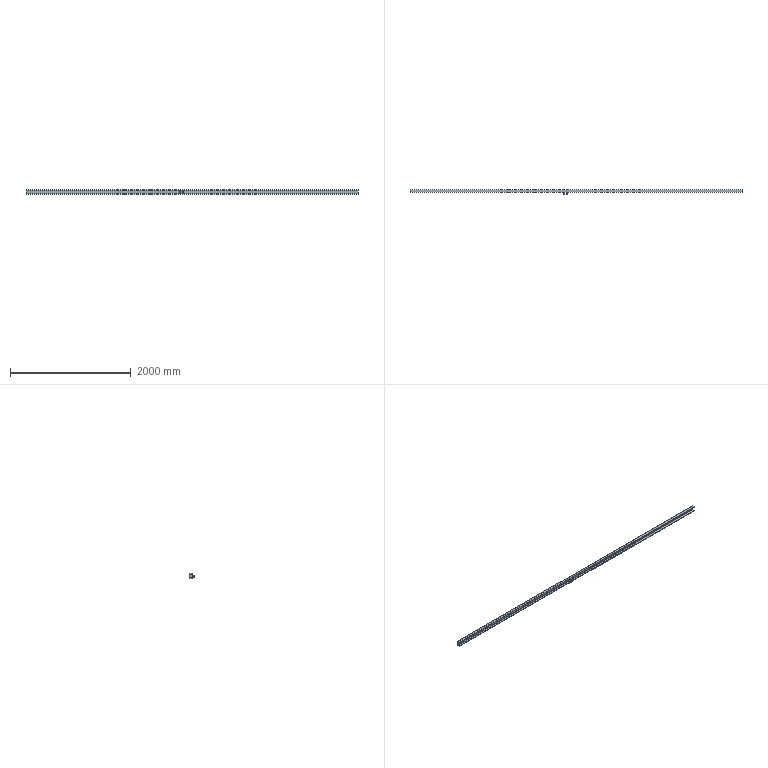Part | STEP file | 3 solids | 36 faces | box 5500 x 77.547 x 80 mm | volume 5816497 mm3 | plane 24 | cylinder 12 | commonest cylinder face diameters 20 x4 40 x4 8 x2 16 x2